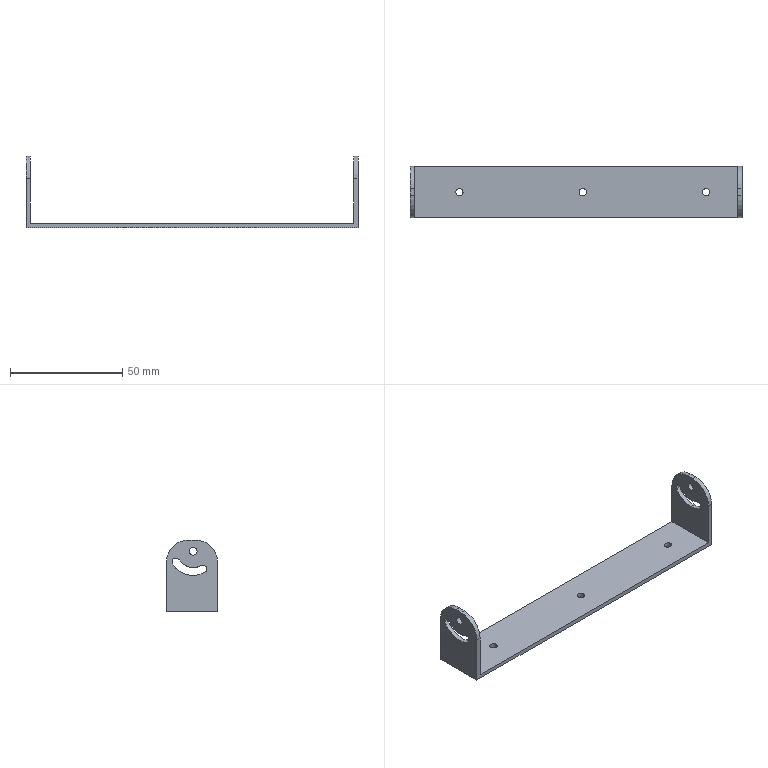Part | STEP file | 11-FG-S00311 | 1 solid | 35 faces | box 148 x 23 x 32 mm | volume 9076 mm3 | cylinder 25 | plane 10 | commonest cylinder face diameters 3.5 x9 3.3 x6 20 x4 14.5 x3 21.5 x3
STEP:
#1=CARTESIAN_POINT('',(18.35,11.492,0.));
#2=VERTEX_POINT('',#1);
#3=CARTESIAN_POINT('',(21.65,11.492,0.));
#4=VERTEX_POINT('',#3);
#5=CARTESIAN_POINT('',(20.,11.492,0.));
#6=DIRECTION('',(0.,0.,1.));
#7=DIRECTION('',(1.,0.,0.));
#8=AXIS2_PLACEMENT_3D('',#5,#6,#7);
#9=CIRCLE('',#8,1.65);
#10=EDGE_CURVE('',#2,#4,#9,.T.);
#11=ORIENTED_EDGE('',*,*,#10,.T.);
#12=CARTESIAN_POINT('',(21.65,11.492,-2.));
#13=VERTEX_POINT('',#12);
#14=CARTESIAN_POINT('',(21.65,11.492,-2.));
#15=DIRECTION('',(0.,0.,-1.));
#16=VECTOR('',#15,1000.);
#17=LINE('',#14,#16);
#18=EDGE_CURVE('',#4,#13,#17,.T.);
#19=ORIENTED_EDGE('',*,*,#18,.T.);
#20=CARTESIAN_POINT('',(18.35,11.492,-2.));
#21=VERTEX_POINT('',#20);
#22=CARTESIAN_POINT('',(20.,11.492,-2.));
#23=DIRECTION('',(0.,0.,-1.));
#24=DIRECTION('',(-1.,0.,0.));
#25=AXIS2_PLACEMENT_3D('',#22,#23,#24);
#26=CIRCLE('',#25,1.65);
#27=EDGE_CURVE('',#13,#21,#26,.T.);
#28=ORIENTED_EDGE('',*,*,#27,.T.);
#29=CARTESIAN_POINT('',(18.35,11.492,-2.));
#30=DIRECTION('',(0.,0.,-1.));
#31=VECTOR('',#30,1000.);
#32=LINE('',#29,#31);
#33=EDGE_CURVE('',#2,#21,#32,.T.);
#34=ORIENTED_EDGE('',*,*,#33,.F.);
#35=EDGE_LOOP('',(#11,#19,#28,#34));
#36=FACE_OUTER_BOUND('',#35,.T.);
#37=CARTESIAN_POINT('',(20.,11.492,-2.));
#38=DIRECTION('',(0.,0.,-1.));
#39=DIRECTION('',(-1.,0.,0.));
#40=AXIS2_PLACEMENT_3D('',#37,#38,#39);
#41=CYLINDRICAL_SURFACE('',#40,1.65);
#42=ADVANCED_FACE('',(#36),#41,.F.);
#43=CARTESIAN_POINT('',(73.35,11.492,0.));
#44=VERTEX_POINT('',#43);
#45=CARTESIAN_POINT('',(76.65,11.492,0.));
#46=VERTEX_POINT('',#45);
#47=CARTESIAN_POINT('',(75.,11.492,0.));
#48=DIRECTION('',(0.,0.,1.));
#49=DIRECTION('',(1.,0.,0.));
#50=AXIS2_PLACEMENT_3D('',#47,#48,#49);
#51=CIRCLE('',#50,1.65);
#52=EDGE_CURVE('',#44,#46,#51,.T.);
#53=ORIENTED_EDGE('',*,*,#52,.T.);
#54=CARTESIAN_POINT('',(76.65,11.492,-2.));
#55=VERTEX_POINT('',#54);
#56=CARTESIAN_POINT('',(76.65,11.492,-2.));
#57=DIRECTION('',(0.,0.,-1.));
#58=VECTOR('',#57,1000.);
#59=LINE('',#56,#58);
#60=EDGE_CURVE('',#46,#55,#59,.T.);
#61=ORIENTED_EDGE('',*,*,#60,.T.);
#62=CARTESIAN_POINT('',(73.35,11.492,-2.));
#63=VERTEX_POINT('',#62);
#64=CARTESIAN_POINT('',(75.,11.492,-2.));
#65=DIRECTION('',(0.,0.,-1.));
#66=DIRECTION('',(-1.,0.,0.));
#67=AXIS2_PLACEMENT_3D('',#64,#65,#66);
#68=CIRCLE('',#67,1.65);
#69=EDGE_CURVE('',#55,#63,#68,.T.);
#70=ORIENTED_EDGE('',*,*,#69,.T.);
#71=CARTESIAN_POINT('',(73.35,11.492,-2.));
#72=DIRECTION('',(0.,0.,-1.));
#73=VECTOR('',#72,1000.);
#74=LINE('',#71,#73);
#75=EDGE_CURVE('',#44,#63,#74,.T.);
#76=ORIENTED_EDGE('',*,*,#75,.F.);
#77=EDGE_LOOP('',(#53,#61,#70,#76));
#78=FACE_OUTER_BOUND('',#77,.T.);
#79=CARTESIAN_POINT('',(75.,11.492,-2.));
#80=DIRECTION('',(0.,0.,-1.));
#81=DIRECTION('',(-1.,0.,0.));
#82=AXIS2_PLACEMENT_3D('',#79,#80,#81);
#83=CYLINDRICAL_SURFACE('',#82,1.65);
#84=ADVANCED_FACE('',(#78),#83,.F.);
#85=CARTESIAN_POINT('',(128.35,11.492,0.));
#86=VERTEX_POINT('',#85);
#87=CARTESIAN_POINT('',(131.65,11.492,0.));
#88=VERTEX_POINT('',#87);
#89=CARTESIAN_POINT('',(130.,11.492,0.));
#90=DIRECTION('',(0.,0.,1.));
#91=DIRECTION('',(1.,0.,0.));
#92=AXIS2_PLACEMENT_3D('',#89,#90,#91);
#93=CIRCLE('',#92,1.65);
#94=EDGE_CURVE('',#86,#88,#93,.T.);
#95=ORIENTED_EDGE('',*,*,#94,.T.);
#96=CARTESIAN_POINT('',(131.65,11.492,-2.));
#97=VERTEX_POINT('',#96);
#98=CARTESIAN_POINT('',(131.65,11.492,-2.));
#99=DIRECTION('',(0.,0.,-1.));
#100=VECTOR('',#99,1000.);
#101=LINE('',#98,#100);
#102=EDGE_CURVE('',#88,#97,#101,.T.);
#103=ORIENTED_EDGE('',*,*,#102,.T.);
#104=CARTESIAN_POINT('',(128.35,11.492,-2.));
#105=VERTEX_POINT('',#104);
#106=CARTESIAN_POINT('',(130.,11.492,-2.));
#107=DIRECTION('',(0.,0.,-1.));
#108=DIRECTION('',(-1.,0.,0.));
#109=AXIS2_PLACEMENT_3D('',#106,#107,#108);
#110=CIRCLE('',#109,1.65);
#111=EDGE_CURVE('',#97,#105,#110,.T.);
#112=ORIENTED_EDGE('',*,*,#111,.T.);
#113=CARTESIAN_POINT('',(128.35,11.492,-2.));
#114=DIRECTION('',(0.,0.,-1.));
#115=VECTOR('',#114,1000.);
#116=LINE('',#113,#115);
#117=EDGE_CURVE('',#86,#105,#116,.T.);
#118=ORIENTED_EDGE('',*,*,#117,.F.);
#119=EDGE_LOOP('',(#95,#103,#112,#118));
#120=FACE_OUTER_BOUND('',#119,.T.);
#121=CARTESIAN_POINT('',(130.,11.492,-2.));
#122=DIRECTION('',(0.,0.,-1.));
#123=DIRECTION('',(-1.,0.,0.));
#124=AXIS2_PLACEMENT_3D('',#121,#122,#123);
#125=CYLINDRICAL_SURFACE('',#124,1.65);
#126=ADVANCED_FACE('',(#120),#125,.F.);
#127=CARTESIAN_POINT('',(144.,11.,17.75));
#128=VERTEX_POINT('',#127);
#129=CARTESIAN_POINT('',(144.,7.501,18.65));
#130=VERTEX_POINT('',#129);
#131=CARTESIAN_POINT('',(144.,11.,25.));
#132=DIRECTION('',(-1.,0.,0.));
#133=DIRECTION('',(0.,0.,-1.));
#134=AXIS2_PLACEMENT_3D('',#131,#132,#133);
#135=CIRCLE('',#134,7.25);
#136=EDGE_CURVE('',#128,#130,#135,.T.);
#137=ORIENTED_EDGE('',*,*,#136,.F.);
#138=CARTESIAN_POINT('',(146.,11.,17.75));
#139=VERTEX_POINT('',#138);
#140=CARTESIAN_POINT('',(144.,11.,17.75));
#141=DIRECTION('',(1.,0.,0.));
#142=VECTOR('',#141,1000.);
#143=LINE('',#140,#142);
#144=EDGE_CURVE('',#128,#139,#143,.T.);
#145=ORIENTED_EDGE('',*,*,#144,.T.);
#146=CARTESIAN_POINT('',(146.,7.501,18.65));
#147=VERTEX_POINT('',#146);
#148=CARTESIAN_POINT('',(146.,11.,25.));
#149=DIRECTION('',(-1.,0.,0.));
#150=DIRECTION('',(0.,0.,-1.));
#151=AXIS2_PLACEMENT_3D('',#148,#149,#150);
#152=CIRCLE('',#151,7.25);
#153=EDGE_CURVE('',#139,#147,#152,.T.);
#154=ORIENTED_EDGE('',*,*,#153,.T.);
#155=CARTESIAN_POINT('',(144.,7.501,18.65));
#156=DIRECTION('',(1.,0.,0.));
#157=VECTOR('',#156,1000.);
#158=LINE('',#155,#157);
#159=EDGE_CURVE('',#130,#147,#158,.T.);
#160=ORIENTED_EDGE('',*,*,#159,.F.);
#161=EDGE_LOOP('',(#137,#145,#154,#160));
#162=FACE_OUTER_BOUND('',#161,.T.);
#163=CARTESIAN_POINT('',(144.,11.,25.));
#164=DIRECTION('',(1.,0.,0.));
#165=DIRECTION('',(0.,0.,-1.));
#166=AXIS2_PLACEMENT_3D('',#163,#164,#165);
#167=CYLINDRICAL_SURFACE('',#166,7.25);
#168=ADVANCED_FACE('',(#162),#167,.T.);
#169=CARTESIAN_POINT('',(144.,11.,14.25));
#170=VERTEX_POINT('',#169);
#171=CARTESIAN_POINT('',(144.,20.15,19.358));
#172=VERTEX_POINT('',#171);
#173=CARTESIAN_POINT('',(144.,11.,25.));
#174=DIRECTION('',(1.,0.,0.));
#175=DIRECTION('',(0.,0.,-1.));
#176=AXIS2_PLACEMENT_3D('',#173,#174,#175);
#177=CIRCLE('',#176,10.75);
#178=EDGE_CURVE('',#170,#172,#177,.T.);
#179=ORIENTED_EDGE('',*,*,#178,.F.);
#180=CARTESIAN_POINT('',(146.,11.,14.25));
#181=VERTEX_POINT('',#180);
#182=CARTESIAN_POINT('',(144.,11.,14.25));
#183=DIRECTION('',(1.,0.,0.));
#184=VECTOR('',#183,1000.);
#185=LINE('',#182,#184);
#186=EDGE_CURVE('',#170,#181,#185,.T.);
#187=ORIENTED_EDGE('',*,*,#186,.T.);
#188=CARTESIAN_POINT('',(146.,20.15,19.358));
#189=VERTEX_POINT('',#188);
#190=CARTESIAN_POINT('',(146.,11.,25.));
#191=DIRECTION('',(1.,0.,0.));
#192=DIRECTION('',(0.,0.,-1.));
#193=AXIS2_PLACEMENT_3D('',#190,#191,#192);
#194=CIRCLE('',#193,10.75);
#195=EDGE_CURVE('',#181,#189,#194,.T.);
#196=ORIENTED_EDGE('',*,*,#195,.T.);
#197=CARTESIAN_POINT('',(144.,20.15,19.358));
#198=DIRECTION('',(1.,0.,0.));
#199=VECTOR('',#198,1000.);
#200=LINE('',#197,#199);
#201=EDGE_CURVE('',#172,#189,#200,.T.);
#202=ORIENTED_EDGE('',*,*,#201,.F.);
#203=EDGE_LOOP('',(#179,#187,#196,#202));
#204=FACE_OUTER_BOUND('',#203,.T.);
#205=CARTESIAN_POINT('',(144.,11.,25.));
#206=DIRECTION('',(1.,0.,0.));
#207=DIRECTION('',(0.,0.,-1.));
#208=AXIS2_PLACEMENT_3D('',#205,#206,#207);
#209=CYLINDRICAL_SURFACE('',#208,10.75);
#210=ADVANCED_FACE('',(#204),#209,.F.);
#211=CARTESIAN_POINT('',(144.,11.,26.75));
#212=VERTEX_POINT('',#211);
#213=CARTESIAN_POINT('',(144.,11.,23.25));
#214=VERTEX_POINT('',#213);
#215=CARTESIAN_POINT('',(144.,11.,25.));
#216=DIRECTION('',(1.,0.,0.));
#217=DIRECTION('',(0.,0.,-1.));
#218=AXIS2_PLACEMENT_3D('',#215,#216,#217);
#219=CIRCLE('',#218,1.75);
#220=EDGE_CURVE('',#212,#214,#219,.T.);
#221=ORIENTED_EDGE('',*,*,#220,.F.);
#222=CARTESIAN_POINT('',(146.,11.,26.75));
#223=VERTEX_POINT('',#222);
#224=CARTESIAN_POINT('',(144.,11.,26.75));
#225=DIRECTION('',(1.,0.,0.));
#226=VECTOR('',#225,1000.);
#227=LINE('',#224,#226);
#228=EDGE_CURVE('',#212,#223,#227,.T.);
#229=ORIENTED_EDGE('',*,*,#228,.T.);
#230=CARTESIAN_POINT('',(146.,11.,23.25));
#231=VERTEX_POINT('',#230);
#232=CARTESIAN_POINT('',(146.,11.,25.));
#233=DIRECTION('',(1.,0.,0.));
#234=DIRECTION('',(0.,0.,-1.));
#235=AXIS2_PLACEMENT_3D('',#232,#233,#234);
#236=CIRCLE('',#235,1.75);
#237=EDGE_CURVE('',#223,#231,#236,.T.);
#238=ORIENTED_EDGE('',*,*,#237,.T.);
#239=CARTESIAN_POINT('',(144.,11.,23.25));
#240=DIRECTION('',(1.,0.,0.));
#241=VECTOR('',#240,1000.);
#242=LINE('',#239,#241);
#243=EDGE_CURVE('',#214,#231,#242,.T.);
#244=ORIENTED_EDGE('',*,*,#243,.F.);
#245=EDGE_LOOP('',(#221,#229,#238,#244));
#246=FACE_OUTER_BOUND('',#245,.T.);
#247=CARTESIAN_POINT('',(144.,11.,25.));
#248=DIRECTION('',(1.,0.,0.));
#249=DIRECTION('',(0.,0.,-1.));
#250=AXIS2_PLACEMENT_3D('',#247,#248,#249);
#251=CYLINDRICAL_SURFACE('',#250,1.75);
#252=ADVANCED_FACE('',(#246),#251,.F.);
#253=CARTESIAN_POINT('',(-2.,20.411,20.276));
#254=VERTEX_POINT('',#253);
#255=CARTESIAN_POINT('',(-2.,17.171,21.195));
#256=VERTEX_POINT('',#255);
#257=CARTESIAN_POINT('',(-2.,18.661,20.276));
#258=DIRECTION('',(1.,0.,0.));
#259=DIRECTION('',(0.,1.,0.));
#260=AXIS2_PLACEMENT_3D('',#257,#258,#259);
#261=CIRCLE('',#260,1.75);
#262=EDGE_CURVE('',#254,#256,#261,.T.);
#263=ORIENTED_EDGE('',*,*,#262,.F.);
#264=CARTESIAN_POINT('',(0.,20.411,20.276));
#265=VERTEX_POINT('',#264);
#266=CARTESIAN_POINT('',(-10.,20.411,20.276));
#267=DIRECTION('',(1.,0.,0.));
#268=VECTOR('',#267,1000.);
#269=LINE('',#266,#268);
#270=EDGE_CURVE('',#254,#265,#269,.T.);
#271=ORIENTED_EDGE('',*,*,#270,.T.);
#272=CARTESIAN_POINT('',(0.,17.171,21.195));
#273=VERTEX_POINT('',#272);
#274=CARTESIAN_POINT('',(0.,18.661,20.276));
#275=DIRECTION('',(1.,0.,0.));
#276=DIRECTION('',(0.,1.,0.));
#277=AXIS2_PLACEMENT_3D('',#274,#275,#276);
#278=CIRCLE('',#277,1.75);
#279=EDGE_CURVE('',#265,#273,#278,.T.);
#280=ORIENTED_EDGE('',*,*,#279,.T.);
#281=CARTESIAN_POINT('',(-10.,17.171,21.195));
#282=DIRECTION('',(1.,0.,0.));
#283=VECTOR('',#282,1000.);
#284=LINE('',#281,#283);
#285=EDGE_CURVE('',#256,#273,#284,.T.);
#286=ORIENTED_EDGE('',*,*,#285,.F.);
#287=EDGE_LOOP('',(#263,#271,#280,#286));
#288=FACE_OUTER_BOUND('',#287,.T.);
#289=CARTESIAN_POINT('',(-10.,18.661,20.276));
#290=DIRECTION('',(1.,0.,0.));
#291=DIRECTION('',(0.,1.,0.));
#292=AXIS2_PLACEMENT_3D('',#289,#290,#291);
#293=CYLINDRICAL_SURFACE('',#292,1.75);
#294=ADVANCED_FACE('',(#288),#293,.F.);
#295=CARTESIAN_POINT('',(-2.,9.25,25.));
#296=VERTEX_POINT('',#295);
#297=CARTESIAN_POINT('',(-2.,12.75,25.));
#298=VERTEX_POINT('',#297);
#299=CARTESIAN_POINT('',(-2.,11.,25.));
#300=DIRECTION('',(1.,0.,0.));
#301=DIRECTION('',(0.,1.,0.));
#302=AXIS2_PLACEMENT_3D('',#299,#300,#301);
#303=CIRCLE('',#302,1.75);
#304=EDGE_CURVE('',#296,#298,#303,.T.);
#305=ORIENTED_EDGE('',*,*,#304,.F.);
#306=CARTESIAN_POINT('',(0.,9.25,25.));
#307=VERTEX_POINT('',#306);
#308=CARTESIAN_POINT('',(-10.,9.25,25.));
#309=DIRECTION('',(1.,0.,0.));
#310=VECTOR('',#309,1000.);
#311=LINE('',#308,#310);
#312=EDGE_CURVE('',#296,#307,#311,.T.);
#313=ORIENTED_EDGE('',*,*,#312,.T.);
#314=CARTESIAN_POINT('',(0.,12.75,25.));
#315=VERTEX_POINT('',#314);
#316=CARTESIAN_POINT('',(0.,11.,25.));
#317=DIRECTION('',(1.,0.,0.));
#318=DIRECTION('',(0.,1.,0.));
#319=AXIS2_PLACEMENT_3D('',#316,#317,#318);
#320=CIRCLE('',#319,1.75);
#321=EDGE_CURVE('',#307,#315,#320,.T.);
#322=ORIENTED_EDGE('',*,*,#321,.T.);
#323=CARTESIAN_POINT('',(-10.,12.75,25.));
#324=DIRECTION('',(1.,0.,0.));
#325=VECTOR('',#324,1000.);
#326=LINE('',#323,#325);
#327=EDGE_CURVE('',#298,#315,#326,.T.);
#328=ORIENTED_EDGE('',*,*,#327,.F.);
#329=EDGE_LOOP('',(#305,#313,#322,#328));
#330=FACE_OUTER_BOUND('',#329,.T.);
#331=CARTESIAN_POINT('',(-10.,11.,25.));
#332=DIRECTION('',(1.,0.,0.));
#333=DIRECTION('',(0.,1.,0.));
#334=AXIS2_PLACEMENT_3D('',#331,#332,#333);
#335=CYLINDRICAL_SURFACE('',#334,1.75);
#336=ADVANCED_FACE('',(#330),#335,.F.);
#337=ORIENTED_EDGE('',*,*,#10,.F.);
#338=CARTESIAN_POINT('',(20.,11.492,0.));
#339=DIRECTION('',(0.,0.,1.));
#340=DIRECTION('',(1.,0.,0.));
#341=AXIS2_PLACEMENT_3D('',#338,#339,#340);
#342=CIRCLE('',#341,1.65);
#343=EDGE_CURVE('',#4,#2,#342,.T.);
#344=ORIENTED_EDGE('',*,*,#343,.F.);
#345=EDGE_LOOP('',(#337,#344));
#346=FACE_BOUND('',#345,.T.);
#347=ORIENTED_EDGE('',*,*,#52,.F.);
#348=CARTESIAN_POINT('',(75.,11.492,0.));
#349=DIRECTION('',(0.,0.,1.));
#350=DIRECTION('',(1.,0.,0.));
#351=AXIS2_PLACEMENT_3D('',#348,#349,#350);
#352=CIRCLE('',#351,1.65);
#353=EDGE_CURVE('',#46,#44,#352,.T.);
#354=ORIENTED_EDGE('',*,*,#353,.F.);
#355=EDGE_LOOP('',(#347,#354));
#356=FACE_BOUND('',#355,.T.);
#357=ORIENTED_EDGE('',*,*,#94,.F.);
#358=CARTESIAN_POINT('',(130.,11.492,0.));
#359=DIRECTION('',(0.,0.,1.));
#360=DIRECTION('',(1.,0.,0.));
#361=AXIS2_PLACEMENT_3D('',#358,#359,#360);
#362=CIRCLE('',#361,1.65);
#363=EDGE_CURVE('',#88,#86,#362,.T.);
#364=ORIENTED_EDGE('',*,*,#363,.F.);
#365=EDGE_LOOP('',(#357,#364));
#366=FACE_BOUND('',#365,.T.);
#367=CARTESIAN_POINT('',(144.,0.,0.));
#368=VERTEX_POINT('',#367);
#369=CARTESIAN_POINT('',(0.,0.,0.));
#370=VERTEX_POINT('',#369);
#371=CARTESIAN_POINT('',(146.,0.,0.));
#372=DIRECTION('',(-1.,0.,0.));
#373=VECTOR('',#372,1000.);
#374=LINE('',#371,#373);
#375=EDGE_CURVE('',#368,#370,#374,.T.);
#376=ORIENTED_EDGE('',*,*,#375,.F.);
#377=CARTESIAN_POINT('',(144.,23.,0.));
#378=VERTEX_POINT('',#377);
#379=CARTESIAN_POINT('',(144.,23.,0.));
#380=DIRECTION('',(0.,1.,0.));
#381=VECTOR('',#380,1000.);
#382=LINE('',#379,#381);
#383=EDGE_CURVE('',#368,#378,#382,.T.);
#384=ORIENTED_EDGE('',*,*,#383,.T.);
#385=CARTESIAN_POINT('',(0.,23.,0.));
#386=VERTEX_POINT('',#385);
#387=CARTESIAN_POINT('',(146.,23.,0.));
#388=DIRECTION('',(1.,0.,0.));
#389=VECTOR('',#388,1000.);
#390=LINE('',#387,#389);
#391=EDGE_CURVE('',#386,#378,#390,.T.);
#392=ORIENTED_EDGE('',*,*,#391,.F.);
#393=CARTESIAN_POINT('',(0.,23.,0.));
#394=DIRECTION('',(0.,-1.,0.));
#395=VECTOR('',#394,1000.);
#396=LINE('',#393,#395);
#397=EDGE_CURVE('',#386,#370,#396,.T.);
#398=ORIENTED_EDGE('',*,*,#397,.T.);
#399=EDGE_LOOP('',(#376,#384,#392,#398));
#400=FACE_OUTER_BOUND('',#399,.T.);
#401=CARTESIAN_POINT('',(0.,0.,0.));
#402=DIRECTION('',(0.,0.,1.));
#403=DIRECTION('',(1.,0.,0.));
#404=AXIS2_PLACEMENT_3D('',#401,#402,#403);
#405=PLANE('',#404);
#406=ADVANCED_FACE('',(#346,#356,#366,#400),#405,.T.);
#407=CARTESIAN_POINT('',(-2.,11.,25.));
#408=DIRECTION('',(1.,0.,0.));
#409=DIRECTION('',(0.,1.,0.));
#410=AXIS2_PLACEMENT_3D('',#407,#408,#409);
#411=CIRCLE('',#410,1.75);
#412=EDGE_CURVE('',#298,#296,#411,.T.);
#413=ORIENTED_EDGE('',*,*,#412,.T.);
#414=ORIENTED_EDGE('',*,*,#304,.T.);
#415=EDGE_LOOP('',(#413,#414));
#416=FACE_BOUND('',#415,.T.);
#417=CARTESIAN_POINT('',(-2.,0.,20.));
#418=VERTEX_POINT('',#417);
#419=CARTESIAN_POINT('',(-2.,0.,-2.));
#420=VERTEX_POINT('',#419);
#421=CARTESIAN_POINT('',(-2.,0.,30.));
#422=DIRECTION('',(0.,0.,-1.));
#423=VECTOR('',#422,1000.);
#424=LINE('',#421,#423);
#425=EDGE_CURVE('',#418,#420,#424,.T.);
#426=ORIENTED_EDGE('',*,*,#425,.F.);
#427=CARTESIAN_POINT('',(-2.,10.,30.));
#428=VERTEX_POINT('',#427);
#429=CARTESIAN_POINT('',(-2.,10.,20.));
#430=DIRECTION('',(-1.,0.,0.));
#431=DIRECTION('',(0.,1.,0.));
#432=AXIS2_PLACEMENT_3D('',#429,#430,#431);
#433=CIRCLE('',#432,10.);
#434=EDGE_CURVE('',#418,#428,#433,.T.);
#435=ORIENTED_EDGE('',*,*,#434,.T.);
#436=CARTESIAN_POINT('',(-2.,13.,30.));
#437=VERTEX_POINT('',#436);
#438=CARTESIAN_POINT('',(-2.,23.,30.));
#439=DIRECTION('',(0.,-1.,0.));
#440=VECTOR('',#439,1000.);
#441=LINE('',#438,#440);
#442=EDGE_CURVE('',#437,#428,#441,.T.);
#443=ORIENTED_EDGE('',*,*,#442,.F.);
#444=CARTESIAN_POINT('',(-2.,23.,20.));
#445=VERTEX_POINT('',#444);
#446=CARTESIAN_POINT('',(-2.,13.,20.));
#447=DIRECTION('',(-1.,0.,0.));
#448=DIRECTION('',(0.,1.,0.));
#449=AXIS2_PLACEMENT_3D('',#446,#447,#448);
#450=CIRCLE('',#449,10.);
#451=EDGE_CURVE('',#437,#445,#450,.T.);
#452=ORIENTED_EDGE('',*,*,#451,.T.);
#453=CARTESIAN_POINT('',(-2.,23.,-2.));
#454=VERTEX_POINT('',#453);
#455=CARTESIAN_POINT('',(-2.,23.,30.));
#456=DIRECTION('',(0.,0.,-1.));
#457=VECTOR('',#456,1000.);
#458=LINE('',#455,#457);
#459=EDGE_CURVE('',#445,#454,#458,.T.);
#460=ORIENTED_EDGE('',*,*,#459,.T.);
#461=CARTESIAN_POINT('',(-2.,0.,-2.));
#462=DIRECTION('',(0.,1.,0.));
#463=VECTOR('',#462,1000.);
#464=LINE('',#461,#463);
#465=EDGE_CURVE('',#420,#454,#464,.T.);
#466=ORIENTED_EDGE('',*,*,#465,.F.);
#467=EDGE_LOOP('',(#426,#435,#443,#452,#460,#466));
#468=FACE_OUTER_BOUND('',#467,.T.);
#469=CARTESIAN_POINT('',(-2.,5.811,15.585));
#470=VERTEX_POINT('',#469);
#471=CARTESIAN_POINT('',(-2.,20.15,19.358));
#472=VERTEX_POINT('',#471);
#473=CARTESIAN_POINT('',(-2.,11.,25.));
#474=DIRECTION('',(1.,0.,0.));
#475=DIRECTION('',(0.,1.,0.));
#476=AXIS2_PLACEMENT_3D('',#473,#474,#475);
#477=CIRCLE('',#476,10.75);
#478=EDGE_CURVE('',#470,#472,#477,.T.);
#479=ORIENTED_EDGE('',*,*,#478,.T.);
#480=CARTESIAN_POINT('',(-2.,18.661,20.276));
#481=DIRECTION('',(1.,0.,0.));
#482=DIRECTION('',(0.,1.,0.));
#483=AXIS2_PLACEMENT_3D('',#480,#481,#482);
#484=CIRCLE('',#483,1.75);
#485=EDGE_CURVE('',#472,#254,#484,.T.);
#486=ORIENTED_EDGE('',*,*,#485,.T.);
#487=ORIENTED_EDGE('',*,*,#262,.T.);
#488=CARTESIAN_POINT('',(-2.,7.501,18.65));
#489=VERTEX_POINT('',#488);
#490=CARTESIAN_POINT('',(-2.,11.,25.));
#491=DIRECTION('',(-1.,0.,0.));
#492=DIRECTION('',(0.,1.,0.));
#493=AXIS2_PLACEMENT_3D('',#490,#491,#492);
#494=CIRCLE('',#493,7.25);
#495=EDGE_CURVE('',#256,#489,#494,.T.);
#496=ORIENTED_EDGE('',*,*,#495,.T.);
#497=CARTESIAN_POINT('',(-2.,6.656,17.118));
#498=DIRECTION('',(1.,0.,0.));
#499=DIRECTION('',(0.,1.,0.));
#500=AXIS2_PLACEMENT_3D('',#497,#498,#499);
#501=CIRCLE('',#500,1.75);
#502=EDGE_CURVE('',#489,#470,#501,.T.);
#503=ORIENTED_EDGE('',*,*,#502,.T.);
#504=EDGE_LOOP('',(#479,#486,#487,#496,#503));
#505=FACE_BOUND('',#504,.T.);
#506=CARTESIAN_POINT('',(-2.,23.,30.));
#507=DIRECTION('',(1.,0.,0.));
#508=DIRECTION('',(0.,1.,0.));
#509=AXIS2_PLACEMENT_3D('',#506,#507,#508);
#510=PLANE('',#509);
#511=ADVANCED_FACE('',(#416,#468,#505),#510,.F.);
#512=CARTESIAN_POINT('',(0.,13.,30.));
#513=VERTEX_POINT('',#512);
#514=CARTESIAN_POINT('',(0.,10.,30.));
#515=VERTEX_POINT('',#514);
#516=CARTESIAN_POINT('',(0.,23.,30.));
#517=DIRECTION('',(0.,-1.,0.));
#518=VECTOR('',#517,1000.);
#519=LINE('',#516,#518);
#520=EDGE_CURVE('',#513,#515,#519,.T.);
#521=ORIENTED_EDGE('',*,*,#520,.T.);
#522=CARTESIAN_POINT('',(0.,0.,20.));
#523=VERTEX_POINT('',#522);
#524=CARTESIAN_POINT('',(0.,10.,20.));
#525=DIRECTION('',(1.,0.,0.));
#526=DIRECTION('',(0.,1.,0.));
#527=AXIS2_PLACEMENT_3D('',#524,#525,#526);
#528=CIRCLE('',#527,10.);
#529=EDGE_CURVE('',#515,#523,#528,.T.);
#530=ORIENTED_EDGE('',*,*,#529,.T.);
#531=CARTESIAN_POINT('',(0.,0.,30.));
#532=DIRECTION('',(0.,0.,-1.));
#533=VECTOR('',#532,1000.);
#534=LINE('',#531,#533);
#535=EDGE_CURVE('',#523,#370,#534,.T.);
#536=ORIENTED_EDGE('',*,*,#535,.T.);
#537=ORIENTED_EDGE('',*,*,#397,.F.);
#538=CARTESIAN_POINT('',(0.,23.,20.));
#539=VERTEX_POINT('',#538);
#540=CARTESIAN_POINT('',(0.,23.,30.));
#541=DIRECTION('',(0.,0.,-1.));
#542=VECTOR('',#541,1000.);
#543=LINE('',#540,#542);
#544=EDGE_CURVE('',#539,#386,#543,.T.);
#545=ORIENTED_EDGE('',*,*,#544,.F.);
#546=CARTESIAN_POINT('',(0.,13.,20.));
#547=DIRECTION('',(1.,0.,0.));
#548=DIRECTION('',(0.,1.,0.));
#549=AXIS2_PLACEMENT_3D('',#546,#547,#548);
#550=CIRCLE('',#549,10.);
#551=EDGE_CURVE('',#539,#513,#550,.T.);
#552=ORIENTED_EDGE('',*,*,#551,.T.);
#553=EDGE_LOOP('',(#521,#530,#536,#537,#545,#552));
#554=FACE_OUTER_BOUND('',#553,.T.);
#555=CARTESIAN_POINT('',(0.,11.,25.));
#556=DIRECTION('',(1.,0.,0.));
#557=DIRECTION('',(0.,1.,0.));
#558=AXIS2_PLACEMENT_3D('',#555,#556,#557);
#559=CIRCLE('',#558,1.75);
#560=EDGE_CURVE('',#315,#307,#559,.T.);
#561=ORIENTED_EDGE('',*,*,#560,.F.);
#562=ORIENTED_EDGE('',*,*,#321,.F.);
#563=EDGE_LOOP('',(#561,#562));
#564=FACE_BOUND('',#563,.T.);
#565=CARTESIAN_POINT('',(0.,20.15,19.358));
#566=VERTEX_POINT('',#565);
#567=CARTESIAN_POINT('',(0.,18.661,20.276));
#568=DIRECTION('',(1.,0.,0.));
#569=DIRECTION('',(0.,1.,0.));
#570=AXIS2_PLACEMENT_3D('',#567,#568,#569);
#571=CIRCLE('',#570,1.75);
#572=EDGE_CURVE('',#566,#265,#571,.T.);
#573=ORIENTED_EDGE('',*,*,#572,.F.);
#574=CARTESIAN_POINT('',(0.,5.811,15.585));
#575=VERTEX_POINT('',#574);
#576=CARTESIAN_POINT('',(0.,11.,25.));
#577=DIRECTION('',(1.,0.,0.));
#578=DIRECTION('',(0.,1.,0.));
#579=AXIS2_PLACEMENT_3D('',#576,#577,#578);
#580=CIRCLE('',#579,10.75);
#581=EDGE_CURVE('',#575,#566,#580,.T.);
#582=ORIENTED_EDGE('',*,*,#581,.F.);
#583=CARTESIAN_POINT('',(0.,7.501,18.65));
#584=VERTEX_POINT('',#583);
#585=CARTESIAN_POINT('',(0.,6.656,17.118));
#586=DIRECTION('',(1.,0.,0.));
#587=DIRECTION('',(0.,1.,0.));
#588=AXIS2_PLACEMENT_3D('',#585,#586,#587);
#589=CIRCLE('',#588,1.75);
#590=EDGE_CURVE('',#584,#575,#589,.T.);
#591=ORIENTED_EDGE('',*,*,#590,.F.);
#592=CARTESIAN_POINT('',(0.,11.,25.));
#593=DIRECTION('',(-1.,0.,0.));
#594=DIRECTION('',(0.,1.,0.));
#595=AXIS2_PLACEMENT_3D('',#592,#593,#594);
#596=CIRCLE('',#595,7.25);
#597=EDGE_CURVE('',#273,#584,#596,.T.);
#598=ORIENTED_EDGE('',*,*,#597,.F.);
#599=ORIENTED_EDGE('',*,*,#279,.F.);
#600=EDGE_LOOP('',(#573,#582,#591,#598,#599));
#601=FACE_BOUND('',#600,.T.);
#602=CARTESIAN_POINT('',(0.,23.,30.));
#603=DIRECTION('',(1.,0.,0.));
#604=DIRECTION('',(0.,1.,0.));
#605=AXIS2_PLACEMENT_3D('',#602,#603,#604);
#606=PLANE('',#605);
#607=ADVANCED_FACE('',(#554,#564,#601),#606,.T.);
#608=ORIENTED_EDGE('',*,*,#535,.F.);
#609=CARTESIAN_POINT('',(-2.,0.,20.));
#610=DIRECTION('',(-1.,0.,0.));
#611=VECTOR('',#610,1000.);
#612=LINE('',#609,#611);
#613=EDGE_CURVE('',#523,#418,#612,.T.);
#614=ORIENTED_EDGE('',*,*,#613,.T.);
#615=ORIENTED_EDGE('',*,*,#425,.T.);
#616=CARTESIAN_POINT('',(146.,0.,-2.));
#617=VERTEX_POINT('',#616);
#618=CARTESIAN_POINT('',(146.,0.,-2.));
#619=DIRECTION('',(-1.,0.,0.));
#620=VECTOR('',#619,1000.);
#621=LINE('',#618,#620);
#622=EDGE_CURVE('',#617,#420,#621,.T.);
#623=ORIENTED_EDGE('',*,*,#622,.F.);
#624=CARTESIAN_POINT('',(146.,0.,20.));
#625=VERTEX_POINT('',#624);
#626=CARTESIAN_POINT('',(146.,0.,-2.));
#627=DIRECTION('',(0.,0.,1.));
#628=VECTOR('',#627,1000.);
#629=LINE('',#626,#628);
#630=EDGE_CURVE('',#617,#625,#629,.T.);
#631=ORIENTED_EDGE('',*,*,#630,.T.);
#632=CARTESIAN_POINT('',(144.,0.,20.));
#633=VERTEX_POINT('',#632);
#634=CARTESIAN_POINT('',(144.,0.,20.));
#635=DIRECTION('',(1.,0.,0.));
#636=VECTOR('',#635,1000.);
#637=LINE('',#634,#636);
#638=EDGE_CURVE('',#633,#625,#637,.T.);
#639=ORIENTED_EDGE('',*,*,#638,.F.);
#640=CARTESIAN_POINT('',(144.,0.,0.));
#641=DIRECTION('',(0.,0.,-1.));
#642=VECTOR('',#641,1000.);
#643=LINE('',#640,#642);
#644=EDGE_CURVE('',#633,#368,#643,.T.);
#645=ORIENTED_EDGE('',*,*,#644,.T.);
#646=ORIENTED_EDGE('',*,*,#375,.T.);
#647=EDGE_LOOP('',(#608,#614,#615,#623,#631,#639,#645,#646));
#648=FACE_OUTER_BOUND('',#647,.T.);
#649=CARTESIAN_POINT('',(0.,0.,30.));
#650=DIRECTION('',(0.,-1.,0.));
#651=DIRECTION('',(0.,0.,-1.));
#652=AXIS2_PLACEMENT_3D('',#649,#650,#651);
#653=PLANE('',#652);
#654=ADVANCED_FACE('',(#648),#653,.T.);
#655=ORIENTED_EDGE('',*,*,#459,.F.);
#656=CARTESIAN_POINT('',(0.,23.,20.));
#657=DIRECTION('',(1.,0.,0.));
#658=VECTOR('',#657,1000.);
#659=LINE('',#656,#658);
#660=EDGE_CURVE('',#445,#539,#659,.T.);
#661=ORIENTED_EDGE('',*,*,#660,.T.);
#662=ORIENTED_EDGE('',*,*,#544,.T.);
#663=ORIENTED_EDGE('',*,*,#391,.T.);
#664=CARTESIAN_POINT('',(144.,23.,20.));
#665=VERTEX_POINT('',#664);
#666=CARTESIAN_POINT('',(144.,23.,0.));
#667=DIRECTION('',(0.,0.,1.));
#668=VECTOR('',#667,1000.);
#669=LINE('',#666,#668);
#670=EDGE_CURVE('',#378,#665,#669,.T.);
#671=ORIENTED_EDGE('',*,*,#670,.T.);
#672=CARTESIAN_POINT('',(146.,23.,20.));
#673=VERTEX_POINT('',#672);
#674=CARTESIAN_POINT('',(144.,23.,20.));
#675=DIRECTION('',(1.,0.,0.));
#676=VECTOR('',#675,1000.);
#677=LINE('',#674,#676);
#678=EDGE_CURVE('',#665,#673,#677,.T.);
#679=ORIENTED_EDGE('',*,*,#678,.T.);
#680=CARTESIAN_POINT('',(146.,23.,-2.));
#681=VERTEX_POINT('',#680);
#682=CARTESIAN_POINT('',(146.,23.,-2.));
#683=DIRECTION('',(0.,0.,1.));
#684=VECTOR('',#683,1000.);
#685=LINE('',#682,#684);
#686=EDGE_CURVE('',#681,#673,#685,.T.);
#687=ORIENTED_EDGE('',*,*,#686,.F.);
#688=CARTESIAN_POINT('',(146.,23.,-2.));
#689=DIRECTION('',(1.,0.,0.));
#690=VECTOR('',#689,1000.);
#691=LINE('',#688,#690);
#692=EDGE_CURVE('',#454,#681,#691,.T.);
#693=ORIENTED_EDGE('',*,*,#692,.F.);
#694=EDGE_LOOP('',(#655,#661,#662,#663,#671,#679,#687,#693));
#695=FACE_OUTER_BOUND('',#694,.T.);
#696=CARTESIAN_POINT('',(-2.,23.,30.));
#697=DIRECTION('',(0.,1.,0.));
#698=DIRECTION('',(0.,0.,1.));
#699=AXIS2_PLACEMENT_3D('',#696,#697,#698);
#700=PLANE('',#699);
#701=ADVANCED_FACE('',(#695),#700,.T.);
#702=ORIENTED_EDGE('',*,*,#442,.T.);
#703=CARTESIAN_POINT('',(0.,10.,30.));
#704=DIRECTION('',(1.,0.,0.));
#705=VECTOR('',#704,1000.);
#706=LINE('',#703,#705);
#707=EDGE_CURVE('',#428,#515,#706,.T.);
#708=ORIENTED_EDGE('',*,*,#707,.T.);
#709=ORIENTED_EDGE('',*,*,#520,.F.);
#710=CARTESIAN_POINT('',(-2.,13.,30.));
#711=DIRECTION('',(-1.,0.,0.));
#712=VECTOR('',#711,1000.);
#713=LINE('',#710,#712);
#714=EDGE_CURVE('',#513,#437,#713,.T.);
#715=ORIENTED_EDGE('',*,*,#714,.T.);
#716=EDGE_LOOP('',(#702,#708,#709,#715));
#717=FACE_OUTER_BOUND('',#716,.T.);
#718=CARTESIAN_POINT('',(0.,0.,30.));
#719=DIRECTION('',(0.,0.,-1.));
#720=DIRECTION('',(-1.,0.,0.));
#721=AXIS2_PLACEMENT_3D('',#718,#719,#720);
#722=PLANE('',#721);
#723=ADVANCED_FACE('',(#717),#722,.F.);
#724=ORIENTED_EDGE('',*,*,#529,.F.);
#725=ORIENTED_EDGE('',*,*,#707,.F.);
#726=ORIENTED_EDGE('',*,*,#434,.F.);
#727=ORIENTED_EDGE('',*,*,#613,.F.);
#728=EDGE_LOOP('',(#724,#725,#726,#727));
#729=FACE_OUTER_BOUND('',#728,.T.);
#730=CARTESIAN_POINT('',(0.,10.,20.));
#731=DIRECTION('',(1.,0.,0.));
#732=DIRECTION('',(0.,0.,-1.));
#733=AXIS2_PLACEMENT_3D('',#730,#731,#732);
#734=CYLINDRICAL_SURFACE('',#733,10.);
#735=ADVANCED_FACE('',(#729),#734,.T.);
#736=ORIENTED_EDGE('',*,*,#451,.F.);
#737=ORIENTED_EDGE('',*,*,#714,.F.);
#738=ORIENTED_EDGE('',*,*,#551,.F.);
#739=ORIENTED_EDGE('',*,*,#660,.F.);
#740=EDGE_LOOP('',(#736,#737,#738,#739));
#741=FACE_OUTER_BOUND('',#740,.T.);
#742=CARTESIAN_POINT('',(-2.,13.,20.));
#743=DIRECTION('',(-1.,0.,0.));
#744=DIRECTION('',(0.,0.,1.));
#745=AXIS2_PLACEMENT_3D('',#742,#743,#744);
#746=CYLINDRICAL_SURFACE('',#745,10.);
#747=ADVANCED_FACE('',(#741),#746,.T.);
#748=ORIENTED_EDGE('',*,*,#312,.F.);
#749=ORIENTED_EDGE('',*,*,#412,.F.);
#750=ORIENTED_EDGE('',*,*,#327,.T.);
#751=ORIENTED_EDGE('',*,*,#560,.T.);
#752=EDGE_LOOP('',(#748,#749,#750,#751));
#753=FACE_OUTER_BOUND('',#752,.T.);
#754=CARTESIAN_POINT('',(-10.,11.,25.));
#755=DIRECTION('',(1.,0.,0.));
#756=DIRECTION('',(0.,1.,0.));
#757=AXIS2_PLACEMENT_3D('',#754,#755,#756);
#758=CYLINDRICAL_SURFACE('',#757,1.75);
#759=ADVANCED_FACE('',(#753),#758,.F.);
#760=ORIENTED_EDGE('',*,*,#270,.F.);
#761=ORIENTED_EDGE('',*,*,#485,.F.);
#762=CARTESIAN_POINT('',(-10.,20.15,19.358));
#763=DIRECTION('',(1.,0.,0.));
#764=VECTOR('',#763,1000.);
#765=LINE('',#762,#764);
#766=EDGE_CURVE('',#472,#566,#765,.T.);
#767=ORIENTED_EDGE('',*,*,#766,.T.);
#768=ORIENTED_EDGE('',*,*,#572,.T.);
#769=EDGE_LOOP('',(#760,#761,#767,#768));
#770=FACE_OUTER_BOUND('',#769,.T.);
#771=CARTESIAN_POINT('',(-10.,18.661,20.276));
#772=DIRECTION('',(1.,0.,0.));
#773=DIRECTION('',(0.,1.,0.));
#774=AXIS2_PLACEMENT_3D('',#771,#772,#773);
#775=CYLINDRICAL_SURFACE('',#774,1.75);
#776=ADVANCED_FACE('',(#770),#775,.F.);
#777=CARTESIAN_POINT('',(-10.,5.811,15.585));
#778=DIRECTION('',(1.,0.,0.));
#779=VECTOR('',#778,1000.);
#780=LINE('',#777,#779);
#781=EDGE_CURVE('',#470,#575,#780,.T.);
#782=ORIENTED_EDGE('',*,*,#781,.T.);
#783=ORIENTED_EDGE('',*,*,#581,.T.);
#784=ORIENTED_EDGE('',*,*,#766,.F.);
#785=ORIENTED_EDGE('',*,*,#478,.F.);
#786=EDGE_LOOP('',(#782,#783,#784,#785));
#787=FACE_OUTER_BOUND('',#786,.T.);
#788=CARTESIAN_POINT('',(-10.,11.,25.));
#789=DIRECTION('',(1.,0.,0.));
#790=DIRECTION('',(0.,1.,0.));
#791=AXIS2_PLACEMENT_3D('',#788,#789,#790);
#792=CYLINDRICAL_SURFACE('',#791,10.75);
#793=ADVANCED_FACE('',(#787),#792,.F.);
#794=CARTESIAN_POINT('',(-10.,7.501,18.65));
#795=DIRECTION('',(1.,0.,0.));
#796=VECTOR('',#795,1000.);
#797=LINE('',#794,#796);
#798=EDGE_CURVE('',#489,#584,#797,.T.);
#799=ORIENTED_EDGE('',*,*,#798,.T.);
#800=ORIENTED_EDGE('',*,*,#590,.T.);
#801=ORIENTED_EDGE('',*,*,#781,.F.);
#802=ORIENTED_EDGE('',*,*,#502,.F.);
#803=EDGE_LOOP('',(#799,#800,#801,#802));
#804=FACE_OUTER_BOUND('',#803,.T.);
#805=CARTESIAN_POINT('',(-10.,6.656,17.118));
#806=DIRECTION('',(1.,0.,0.));
#807=DIRECTION('',(0.,1.,0.));
#808=AXIS2_PLACEMENT_3D('',#805,#806,#807);
#809=CYLINDRICAL_SURFACE('',#808,1.75);
#810=ADVANCED_FACE('',(#804),#809,.F.);
#811=ORIENTED_EDGE('',*,*,#285,.T.);
#812=ORIENTED_EDGE('',*,*,#597,.T.);
#813=ORIENTED_EDGE('',*,*,#798,.F.);
#814=ORIENTED_EDGE('',*,*,#495,.F.);
#815=EDGE_LOOP('',(#811,#812,#813,#814));
#816=FACE_OUTER_BOUND('',#815,.T.);
#817=CARTESIAN_POINT('',(-10.,11.,25.));
#818=DIRECTION('',(1.,0.,0.));
#819=DIRECTION('',(0.,1.,0.));
#820=AXIS2_PLACEMENT_3D('',#817,#818,#819);
#821=CYLINDRICAL_SURFACE('',#820,7.25);
#822=ADVANCED_FACE('',(#816),#821,.T.);
#823=ORIENTED_EDGE('',*,*,#686,.T.);
#824=CARTESIAN_POINT('',(146.,13.,30.));
#825=VERTEX_POINT('',#824);
#826=CARTESIAN_POINT('',(146.,13.,20.));
#827=DIRECTION('',(1.,0.,0.));
#828=DIRECTION('',(0.,0.,-1.));
#829=AXIS2_PLACEMENT_3D('',#826,#827,#828);
#830=CIRCLE('',#829,10.);
#831=EDGE_CURVE('',#673,#825,#830,.T.);
#832=ORIENTED_EDGE('',*,*,#831,.T.);
#833=CARTESIAN_POINT('',(146.,10.,30.));
#834=VERTEX_POINT('',#833);
#835=CARTESIAN_POINT('',(146.,13.,30.));
#836=DIRECTION('',(0.,-1.,0.));
#837=VECTOR('',#836,1000.);
#838=LINE('',#835,#837);
#839=EDGE_CURVE('',#825,#834,#838,.T.);
#840=ORIENTED_EDGE('',*,*,#839,.T.);
#841=CARTESIAN_POINT('',(146.,10.,20.));
#842=DIRECTION('',(1.,0.,0.));
#843=DIRECTION('',(0.,0.,-1.));
#844=AXIS2_PLACEMENT_3D('',#841,#842,#843);
#845=CIRCLE('',#844,10.);
#846=EDGE_CURVE('',#834,#625,#845,.T.);
#847=ORIENTED_EDGE('',*,*,#846,.T.);
#848=ORIENTED_EDGE('',*,*,#630,.F.);
#849=CARTESIAN_POINT('',(146.,0.,-2.));
#850=DIRECTION('',(0.,-1.,0.));
#851=VECTOR('',#850,1000.);
#852=LINE('',#849,#851);
#853=EDGE_CURVE('',#681,#617,#852,.T.);
#854=ORIENTED_EDGE('',*,*,#853,.F.);
#855=EDGE_LOOP('',(#823,#832,#840,#847,#848,#854));
#856=FACE_OUTER_BOUND('',#855,.T.);
#857=CARTESIAN_POINT('',(146.,5.811,15.585));
#858=VERTEX_POINT('',#857);
#859=CARTESIAN_POINT('',(146.,11.,25.));
#860=DIRECTION('',(1.,0.,0.));
#861=DIRECTION('',(0.,0.,-1.));
#862=AXIS2_PLACEMENT_3D('',#859,#860,#861);
#863=CIRCLE('',#862,10.75);
#864=EDGE_CURVE('',#858,#181,#863,.T.);
#865=ORIENTED_EDGE('',*,*,#864,.F.);
#866=CARTESIAN_POINT('',(146.,6.656,17.118));
#867=DIRECTION('',(1.,0.,0.));
#868=DIRECTION('',(0.,0.,-1.));
#869=AXIS2_PLACEMENT_3D('',#866,#867,#868);
#870=CIRCLE('',#869,1.75);
#871=EDGE_CURVE('',#147,#858,#870,.T.);
#872=ORIENTED_EDGE('',*,*,#871,.F.);
#873=ORIENTED_EDGE('',*,*,#153,.F.);
#874=CARTESIAN_POINT('',(146.,17.171,21.195));
#875=VERTEX_POINT('',#874);
#876=CARTESIAN_POINT('',(146.,11.,25.));
#877=DIRECTION('',(-1.,0.,0.));
#878=DIRECTION('',(0.,0.,-1.));
#879=AXIS2_PLACEMENT_3D('',#876,#877,#878);
#880=CIRCLE('',#879,7.25);
#881=EDGE_CURVE('',#875,#139,#880,.T.);
#882=ORIENTED_EDGE('',*,*,#881,.F.);
#883=CARTESIAN_POINT('',(146.,18.661,20.276));
#884=DIRECTION('',(1.,0.,0.));
#885=DIRECTION('',(0.,0.,-1.));
#886=AXIS2_PLACEMENT_3D('',#883,#884,#885);
#887=CIRCLE('',#886,1.75);
#888=EDGE_CURVE('',#189,#875,#887,.T.);
#889=ORIENTED_EDGE('',*,*,#888,.F.);
#890=ORIENTED_EDGE('',*,*,#195,.F.);
#891=EDGE_LOOP('',(#865,#872,#873,#882,#889,#890));
#892=FACE_BOUND('',#891,.T.);
#893=CARTESIAN_POINT('',(146.,11.,25.));
#894=DIRECTION('',(1.,0.,0.));
#895=DIRECTION('',(0.,0.,-1.));
#896=AXIS2_PLACEMENT_3D('',#893,#894,#895);
#897=CIRCLE('',#896,1.75);
#898=EDGE_CURVE('',#231,#223,#897,.T.);
#899=ORIENTED_EDGE('',*,*,#898,.F.);
#900=ORIENTED_EDGE('',*,*,#237,.F.);
#901=EDGE_LOOP('',(#899,#900));
#902=FACE_BOUND('',#901,.T.);
#903=CARTESIAN_POINT('',(146.,0.,-2.));
#904=DIRECTION('',(-1.,0.,0.));
#905=DIRECTION('',(0.,0.,1.));
#906=AXIS2_PLACEMENT_3D('',#903,#904,#905);
#907=PLANE('',#906);
#908=ADVANCED_FACE('',(#856,#892,#902),#907,.F.);
#909=CARTESIAN_POINT('',(20.,11.492,-2.));
#910=DIRECTION('',(0.,0.,-1.));
#911=DIRECTION('',(-1.,0.,0.));
#912=AXIS2_PLACEMENT_3D('',#909,#910,#911);
#913=CIRCLE('',#912,1.65);
#914=EDGE_CURVE('',#21,#13,#913,.T.);
#915=ORIENTED_EDGE('',*,*,#914,.F.);
#916=ORIENTED_EDGE('',*,*,#27,.F.);
#917=EDGE_LOOP('',(#915,#916));
#918=FACE_BOUND('',#917,.T.);
#919=CARTESIAN_POINT('',(75.,11.492,-2.));
#920=DIRECTION('',(0.,0.,-1.));
#921=DIRECTION('',(-1.,0.,0.));
#922=AXIS2_PLACEMENT_3D('',#919,#920,#921);
#923=CIRCLE('',#922,1.65);
#924=EDGE_CURVE('',#63,#55,#923,.T.);
#925=ORIENTED_EDGE('',*,*,#924,.F.);
#926=ORIENTED_EDGE('',*,*,#69,.F.);
#927=EDGE_LOOP('',(#925,#926));
#928=FACE_BOUND('',#927,.T.);
#929=CARTESIAN_POINT('',(130.,11.492,-2.));
#930=DIRECTION('',(0.,0.,-1.));
#931=DIRECTION('',(-1.,0.,0.));
#932=AXIS2_PLACEMENT_3D('',#929,#930,#931);
#933=CIRCLE('',#932,1.65);
#934=EDGE_CURVE('',#105,#97,#933,.T.);
#935=ORIENTED_EDGE('',*,*,#934,.F.);
#936=ORIENTED_EDGE('',*,*,#111,.F.);
#937=EDGE_LOOP('',(#935,#936));
#938=FACE_BOUND('',#937,.T.);
#939=ORIENTED_EDGE('',*,*,#853,.T.);
#940=ORIENTED_EDGE('',*,*,#622,.T.);
#941=ORIENTED_EDGE('',*,*,#465,.T.);
#942=ORIENTED_EDGE('',*,*,#692,.T.);
#943=EDGE_LOOP('',(#939,#940,#941,#942));
#944=FACE_OUTER_BOUND('',#943,.T.);
#945=CARTESIAN_POINT('',(0.,0.,-2.));
#946=DIRECTION('',(0.,0.,1.));
#947=DIRECTION('',(1.,0.,0.));
#948=AXIS2_PLACEMENT_3D('',#945,#946,#947);
#949=PLANE('',#948);
#950=ADVANCED_FACE('',(#918,#928,#938,#944),#949,.F.);
#951=ORIENTED_EDGE('',*,*,#846,.F.);
#952=CARTESIAN_POINT('',(144.,10.,30.));
#953=VERTEX_POINT('',#952);
#954=CARTESIAN_POINT('',(144.,10.,30.));
#955=DIRECTION('',(1.,0.,0.));
#956=VECTOR('',#955,1000.);
#957=LINE('',#954,#956);
#958=EDGE_CURVE('',#953,#834,#957,.T.);
#959=ORIENTED_EDGE('',*,*,#958,.F.);
#960=CARTESIAN_POINT('',(144.,10.,20.));
#961=DIRECTION('',(1.,0.,0.));
#962=DIRECTION('',(0.,0.,-1.));
#963=AXIS2_PLACEMENT_3D('',#960,#961,#962);
#964=CIRCLE('',#963,10.);
#965=EDGE_CURVE('',#953,#633,#964,.T.);
#966=ORIENTED_EDGE('',*,*,#965,.T.);
#967=ORIENTED_EDGE('',*,*,#638,.T.);
#968=EDGE_LOOP('',(#951,#959,#966,#967));
#969=FACE_OUTER_BOUND('',#968,.T.);
#970=CARTESIAN_POINT('',(144.,10.,20.));
#971=DIRECTION('',(1.,0.,0.));
#972=DIRECTION('',(0.,0.,-1.));
#973=AXIS2_PLACEMENT_3D('',#970,#971,#972);
#974=CYLINDRICAL_SURFACE('',#973,10.);
#975=ADVANCED_FACE('',(#969),#974,.T.);
#976=ORIENTED_EDGE('',*,*,#839,.F.);
#977=CARTESIAN_POINT('',(144.,13.,30.));
#978=VERTEX_POINT('',#977);
#979=CARTESIAN_POINT('',(144.,13.,30.));
#980=DIRECTION('',(1.,0.,0.));
#981=VECTOR('',#980,1000.);
#982=LINE('',#979,#981);
#983=EDGE_CURVE('',#978,#825,#982,.T.);
#984=ORIENTED_EDGE('',*,*,#983,.F.);
#985=CARTESIAN_POINT('',(144.,13.,30.));
#986=DIRECTION('',(0.,-1.,0.));
#987=VECTOR('',#986,1000.);
#988=LINE('',#985,#987);
#989=EDGE_CURVE('',#978,#953,#988,.T.);
#990=ORIENTED_EDGE('',*,*,#989,.T.);
#991=ORIENTED_EDGE('',*,*,#958,.T.);
#992=EDGE_LOOP('',(#976,#984,#990,#991));
#993=FACE_OUTER_BOUND('',#992,.T.);
#994=CARTESIAN_POINT('',(144.,13.,30.));
#995=DIRECTION('',(0.,0.,1.));
#996=DIRECTION('',(0.,-1.,0.));
#997=AXIS2_PLACEMENT_3D('',#994,#995,#996);
#998=PLANE('',#997);
#999=ADVANCED_FACE('',(#993),#998,.T.);
#1000=ORIENTED_EDGE('',*,*,#831,.F.);
#1001=ORIENTED_EDGE('',*,*,#678,.F.);
#1002=CARTESIAN_POINT('',(144.,13.,20.));
#1003=DIRECTION('',(1.,0.,0.));
#1004=DIRECTION('',(0.,0.,-1.));
#1005=AXIS2_PLACEMENT_3D('',#1002,#1003,#1004);
#1006=CIRCLE('',#1005,10.);
#1007=EDGE_CURVE('',#665,#978,#1006,.T.);
#1008=ORIENTED_EDGE('',*,*,#1007,.T.);
#1009=ORIENTED_EDGE('',*,*,#983,.T.);
#1010=EDGE_LOOP('',(#1000,#1001,#1008,#1009));
#1011=FACE_OUTER_BOUND('',#1010,.T.);
#1012=CARTESIAN_POINT('',(144.,13.,20.));
#1013=DIRECTION('',(1.,0.,0.));
#1014=DIRECTION('',(0.,0.,-1.));
#1015=AXIS2_PLACEMENT_3D('',#1012,#1013,#1014);
#1016=CYLINDRICAL_SURFACE('',#1015,10.);
#1017=ADVANCED_FACE('',(#1011),#1016,.T.);
#1018=CARTESIAN_POINT('',(144.,5.811,15.585));
#1019=VERTEX_POINT('',#1018);
#1020=CARTESIAN_POINT('',(144.,6.656,17.118));
#1021=DIRECTION('',(1.,0.,0.));
#1022=DIRECTION('',(0.,0.,-1.));
#1023=AXIS2_PLACEMENT_3D('',#1020,#1021,#1022);
#1024=CIRCLE('',#1023,1.75);
#1025=EDGE_CURVE('',#130,#1019,#1024,.T.);
#1026=ORIENTED_EDGE('',*,*,#1025,.T.);
#1027=CARTESIAN_POINT('',(144.,11.,25.));
#1028=DIRECTION('',(1.,0.,0.));
#1029=DIRECTION('',(0.,0.,-1.));
#1030=AXIS2_PLACEMENT_3D('',#1027,#1028,#1029);
#1031=CIRCLE('',#1030,10.75);
#1032=EDGE_CURVE('',#1019,#170,#1031,.T.);
#1033=ORIENTED_EDGE('',*,*,#1032,.T.);
#1034=ORIENTED_EDGE('',*,*,#178,.T.);
#1035=CARTESIAN_POINT('',(144.,17.171,21.195));
#1036=VERTEX_POINT('',#1035);
#1037=CARTESIAN_POINT('',(144.,18.661,20.276));
#1038=DIRECTION('',(1.,0.,0.));
#1039=DIRECTION('',(0.,0.,-1.));
#1040=AXIS2_PLACEMENT_3D('',#1037,#1038,#1039);
#1041=CIRCLE('',#1040,1.75);
#1042=EDGE_CURVE('',#172,#1036,#1041,.T.);
#1043=ORIENTED_EDGE('',*,*,#1042,.T.);
#1044=CARTESIAN_POINT('',(144.,11.,25.));
#1045=DIRECTION('',(-1.,0.,0.));
#1046=DIRECTION('',(0.,0.,-1.));
#1047=AXIS2_PLACEMENT_3D('',#1044,#1045,#1046);
#1048=CIRCLE('',#1047,7.25);
#1049=EDGE_CURVE('',#1036,#128,#1048,.T.);
#1050=ORIENTED_EDGE('',*,*,#1049,.T.);
#1051=ORIENTED_EDGE('',*,*,#136,.T.);
#1052=EDGE_LOOP('',(#1026,#1033,#1034,#1043,#1050,#1051));
#1053=FACE_BOUND('',#1052,.T.);
#1054=CARTESIAN_POINT('',(144.,11.,25.));
#1055=DIRECTION('',(1.,0.,0.));
#1056=DIRECTION('',(0.,0.,-1.));
#1057=AXIS2_PLACEMENT_3D('',#1054,#1055,#1056);
#1058=CIRCLE('',#1057,1.75);
#1059=EDGE_CURVE('',#214,#212,#1058,.T.);
#1060=ORIENTED_EDGE('',*,*,#1059,.T.);
#1061=ORIENTED_EDGE('',*,*,#220,.T.);
#1062=EDGE_LOOP('',(#1060,#1061));
#1063=FACE_BOUND('',#1062,.T.);
#1064=ORIENTED_EDGE('',*,*,#383,.F.);
#1065=ORIENTED_EDGE('',*,*,#644,.F.);
#1066=ORIENTED_EDGE('',*,*,#965,.F.);
#1067=ORIENTED_EDGE('',*,*,#989,.F.);
#1068=ORIENTED_EDGE('',*,*,#1007,.F.);
#1069=ORIENTED_EDGE('',*,*,#670,.F.);
#1070=EDGE_LOOP('',(#1064,#1065,#1066,#1067,#1068,#1069));
#1071=FACE_OUTER_BOUND('',#1070,.T.);
#1072=CARTESIAN_POINT('',(144.,10.,20.));
#1073=DIRECTION('',(1.,0.,0.));
#1074=DIRECTION('',(0.,0.,-1.));
#1075=AXIS2_PLACEMENT_3D('',#1072,#1073,#1074);
#1076=PLANE('',#1075);
#1077=ADVANCED_FACE('',(#1053,#1063,#1071),#1076,.F.);
#1078=ORIENTED_EDGE('',*,*,#228,.F.);
#1079=ORIENTED_EDGE('',*,*,#1059,.F.);
#1080=ORIENTED_EDGE('',*,*,#243,.T.);
#1081=ORIENTED_EDGE('',*,*,#898,.T.);
#1082=EDGE_LOOP('',(#1078,#1079,#1080,#1081));
#1083=FACE_OUTER_BOUND('',#1082,.T.);
#1084=CARTESIAN_POINT('',(144.,11.,25.));
#1085=DIRECTION('',(1.,0.,0.));
#1086=DIRECTION('',(0.,0.,-1.));
#1087=AXIS2_PLACEMENT_3D('',#1084,#1085,#1086);
#1088=CYLINDRICAL_SURFACE('',#1087,1.75);
#1089=ADVANCED_FACE('',(#1083),#1088,.F.);
#1090=ORIENTED_EDGE('',*,*,#186,.F.);
#1091=ORIENTED_EDGE('',*,*,#1032,.F.);
#1092=CARTESIAN_POINT('',(144.,5.811,15.585));
#1093=DIRECTION('',(1.,0.,0.));
#1094=VECTOR('',#1093,1000.);
#1095=LINE('',#1092,#1094);
#1096=EDGE_CURVE('',#1019,#858,#1095,.T.);
#1097=ORIENTED_EDGE('',*,*,#1096,.T.);
#1098=ORIENTED_EDGE('',*,*,#864,.T.);
#1099=EDGE_LOOP('',(#1090,#1091,#1097,#1098));
#1100=FACE_OUTER_BOUND('',#1099,.T.);
#1101=CARTESIAN_POINT('',(144.,11.,25.));
#1102=DIRECTION('',(1.,0.,0.));
#1103=DIRECTION('',(0.,0.,-1.));
#1104=AXIS2_PLACEMENT_3D('',#1101,#1102,#1103);
#1105=CYLINDRICAL_SURFACE('',#1104,10.75);
#1106=ADVANCED_FACE('',(#1100),#1105,.F.);
#1107=ORIENTED_EDGE('',*,*,#871,.T.);
#1108=ORIENTED_EDGE('',*,*,#1096,.F.);
#1109=ORIENTED_EDGE('',*,*,#1025,.F.);
#1110=ORIENTED_EDGE('',*,*,#159,.T.);
#1111=EDGE_LOOP('',(#1107,#1108,#1109,#1110));
#1112=FACE_OUTER_BOUND('',#1111,.T.);
#1113=CARTESIAN_POINT('',(144.,6.656,17.118));
#1114=DIRECTION('',(1.,0.,0.));
#1115=DIRECTION('',(0.,0.,-1.));
#1116=AXIS2_PLACEMENT_3D('',#1113,#1114,#1115);
#1117=CYLINDRICAL_SURFACE('',#1116,1.75);
#1118=ADVANCED_FACE('',(#1112),#1117,.F.);
#1119=ORIENTED_EDGE('',*,*,#144,.F.);
#1120=ORIENTED_EDGE('',*,*,#1049,.F.);
#1121=CARTESIAN_POINT('',(144.,17.171,21.195));
#1122=DIRECTION('',(1.,0.,0.));
#1123=VECTOR('',#1122,1000.);
#1124=LINE('',#1121,#1123);
#1125=EDGE_CURVE('',#1036,#875,#1124,.T.);
#1126=ORIENTED_EDGE('',*,*,#1125,.T.);
#1127=ORIENTED_EDGE('',*,*,#881,.T.);
#1128=EDGE_LOOP('',(#1119,#1120,#1126,#1127));
#1129=FACE_OUTER_BOUND('',#1128,.T.);
#1130=CARTESIAN_POINT('',(144.,11.,25.));
#1131=DIRECTION('',(1.,0.,0.));
#1132=DIRECTION('',(0.,0.,-1.));
#1133=AXIS2_PLACEMENT_3D('',#1130,#1131,#1132);
#1134=CYLINDRICAL_SURFACE('',#1133,7.25);
#1135=ADVANCED_FACE('',(#1129),#1134,.T.);
#1136=ORIENTED_EDGE('',*,*,#888,.T.);
#1137=ORIENTED_EDGE('',*,*,#1125,.F.);
#1138=ORIENTED_EDGE('',*,*,#1042,.F.);
#1139=ORIENTED_EDGE('',*,*,#201,.T.);
#1140=EDGE_LOOP('',(#1136,#1137,#1138,#1139));
#1141=FACE_OUTER_BOUND('',#1140,.T.);
#1142=CARTESIAN_POINT('',(144.,18.661,20.276));
#1143=DIRECTION('',(1.,0.,0.));
#1144=DIRECTION('',(0.,0.,-1.));
#1145=AXIS2_PLACEMENT_3D('',#1142,#1143,#1144);
#1146=CYLINDRICAL_SURFACE('',#1145,1.75);
#1147=ADVANCED_FACE('',(#1141),#1146,.F.);
#1148=ORIENTED_EDGE('',*,*,#102,.F.);
#1149=ORIENTED_EDGE('',*,*,#363,.T.);
#1150=ORIENTED_EDGE('',*,*,#117,.T.);
#1151=ORIENTED_EDGE('',*,*,#934,.T.);
#1152=EDGE_LOOP('',(#1148,#1149,#1150,#1151));
#1153=FACE_OUTER_BOUND('',#1152,.T.);
#1154=CARTESIAN_POINT('',(130.,11.492,-2.));
#1155=DIRECTION('',(0.,0.,-1.));
#1156=DIRECTION('',(-1.,0.,0.));
#1157=AXIS2_PLACEMENT_3D('',#1154,#1155,#1156);
#1158=CYLINDRICAL_SURFACE('',#1157,1.65);
#1159=ADVANCED_FACE('',(#1153),#1158,.F.);
#1160=ORIENTED_EDGE('',*,*,#60,.F.);
#1161=ORIENTED_EDGE('',*,*,#353,.T.);
#1162=ORIENTED_EDGE('',*,*,#75,.T.);
#1163=ORIENTED_EDGE('',*,*,#924,.T.);
#1164=EDGE_LOOP('',(#1160,#1161,#1162,#1163));
#1165=FACE_OUTER_BOUND('',#1164,.T.);
#1166=CARTESIAN_POINT('',(75.,11.492,-2.));
#1167=DIRECTION('',(0.,0.,-1.));
#1168=DIRECTION('',(-1.,0.,0.));
#1169=AXIS2_PLACEMENT_3D('',#1166,#1167,#1168);
#1170=CYLINDRICAL_SURFACE('',#1169,1.65);
#1171=ADVANCED_FACE('',(#1165),#1170,.F.);
#1172=ORIENTED_EDGE('',*,*,#18,.F.);
#1173=ORIENTED_EDGE('',*,*,#343,.T.);
#1174=ORIENTED_EDGE('',*,*,#33,.T.);
#1175=ORIENTED_EDGE('',*,*,#914,.T.);
#1176=EDGE_LOOP('',(#1172,#1173,#1174,#1175));
#1177=FACE_OUTER_BOUND('',#1176,.T.);
#1178=CARTESIAN_POINT('',(20.,11.492,-2.));
#1179=DIRECTION('',(0.,0.,-1.));
#1180=DIRECTION('',(-1.,0.,0.));
#1181=AXIS2_PLACEMENT_3D('',#1178,#1179,#1180);
#1182=CYLINDRICAL_SURFACE('',#1181,1.65);
#1183=ADVANCED_FACE('',(#1177),#1182,.F.);
#1184=CLOSED_SHELL('',(#42,#84,#126,#168,#210,#252,#294,#336,#406,#511,#607,#654,#701,#723,#735,#747,#759,#776,#793,#810,#822,#908,#950,#975,#999,#1017,#1077,#1089,#1106,#1118,#1135,#1147,#1159,#1171,#1183));
#1185=MANIFOLD_SOLID_BREP('',#1184);
#1186=CARTESIAN_POINT('',(0.,0.,0.));
#1187=DIRECTION('',(0.,0.,1.));
#1188=DIRECTION('',(1.,0.,0.));
#1189=AXIS2_PLACEMENT_3D('',#1186,#1187,#1188);
#1190=(LENGTH_UNIT()NAMED_UNIT(*)SI_UNIT(.MILLI.,.METRE.));
#1191=UNCERTAINTY_MEASURE_WITH_UNIT(LENGTH_MEASURE(0.00001),#1190,'','');
#1192=(NAMED_UNIT(*)PLANE_ANGLE_UNIT()SI_UNIT($,.RADIAN.));
#1193=(NAMED_UNIT(*)SI_UNIT($,.STERADIAN.)SOLID_ANGLE_UNIT());
#1194=(GEOMETRIC_REPRESENTATION_CONTEXT(3)GLOBAL_UNCERTAINTY_ASSIGNED_CONTEXT((#1191))GLOBAL_UNIT_ASSIGNED_CONTEXT((#1190,#1192,#1193))REPRESENTATION_CONTEXT('',''));
#1195=ADVANCED_BREP_SHAPE_REPRESENTATION('',(#1185,#1189),#1194);